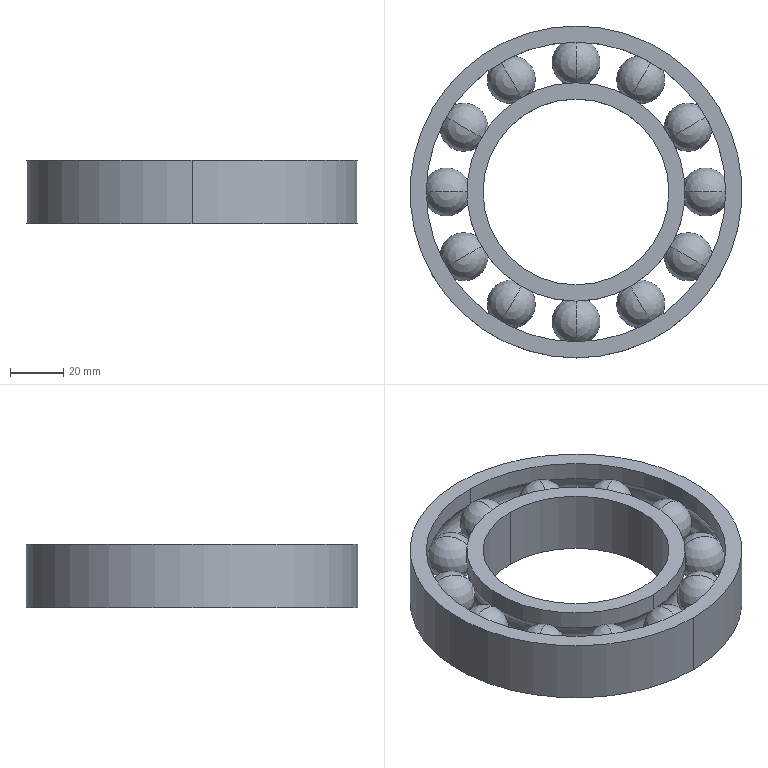Part | NX | features BREP 14 | 14 solids | 44 faces | box 125 x 125 x 24 mm | volume 122130 mm3 | sphere 24 | cylinder 12 | plane 4 | torus 4 | commonest cylinder face diameters 82.222 x4 112.778 x4 70 x2 125 x2
STEP:
#1=CARTESIAN_POINT('',(0.,62.5,-12.));
#2=VERTEX_POINT('',#1);
#3=CARTESIAN_POINT('',(0.,-62.5,-12.));
#4=VERTEX_POINT('',#3);
#5=CARTESIAN_POINT('',(0.,0.,-12.));
#6=DIRECTION('',(0.,0.,1.));
#7=DIRECTION('',(0.,1.,0.));
#8=AXIS2_PLACEMENT_3D('',#5,#6,#7);
#9=CIRCLE('',#8,62.5);
#10=EDGE_CURVE('',#2,#4,#9,.T.);
#11=ORIENTED_EDGE('',*,*,#10,.T.);
#12=CARTESIAN_POINT('',(0.,-62.5,12.));
#13=VERTEX_POINT('',#12);
#14=CARTESIAN_POINT('',(0.,-62.5,-12.));
#15=DIRECTION('',(0.,0.,1.));
#16=VECTOR('',#15,1000.);
#17=LINE('',#14,#16);
#18=EDGE_CURVE('',#4,#13,#17,.T.);
#19=ORIENTED_EDGE('',*,*,#18,.T.);
#20=CARTESIAN_POINT('',(0.,62.5,12.));
#21=VERTEX_POINT('',#20);
#22=CARTESIAN_POINT('',(0.,0.,12.));
#23=DIRECTION('',(0.,0.,1.));
#24=DIRECTION('',(0.,1.,0.));
#25=AXIS2_PLACEMENT_3D('',#22,#23,#24);
#26=CIRCLE('',#25,62.5);
#27=EDGE_CURVE('',#21,#13,#26,.T.);
#28=ORIENTED_EDGE('',*,*,#27,.F.);
#29=CARTESIAN_POINT('',(0.,62.5,-12.));
#30=DIRECTION('',(0.,0.,1.));
#31=VECTOR('',#30,1000.);
#32=LINE('',#29,#31);
#33=EDGE_CURVE('',#2,#21,#32,.T.);
#34=ORIENTED_EDGE('',*,*,#33,.F.);
#35=EDGE_LOOP('',(#11,#19,#28,#34));
#36=FACE_BOUND('',#35,.T.);
#37=CARTESIAN_POINT('',(0.,0.,13.2));
#38=DIRECTION('',(0.,0.,-1.));
#39=DIRECTION('',(0.,1.,0.));
#40=AXIS2_PLACEMENT_3D('',#37,#38,#39);
#41=CYLINDRICAL_SURFACE('',#40,62.5);
#42=ADVANCED_FACE('',(#36),#41,.T.);
#43=CARTESIAN_POINT('',(0.,0.,12.));
#44=DIRECTION('',(0.,0.,-1.));
#45=DIRECTION('',(0.,1.,0.));
#46=AXIS2_PLACEMENT_3D('',#43,#44,#45);
#47=CIRCLE('',#46,62.5);
#48=EDGE_CURVE('',#21,#13,#47,.T.);
#49=ORIENTED_EDGE('',*,*,#48,.T.);
#50=ORIENTED_EDGE('',*,*,#18,.F.);
#51=CARTESIAN_POINT('',(0.,0.,-12.));
#52=DIRECTION('',(0.,0.,-1.));
#53=DIRECTION('',(0.,1.,0.));
#54=AXIS2_PLACEMENT_3D('',#51,#52,#53);
#55=CIRCLE('',#54,62.5);
#56=EDGE_CURVE('',#2,#4,#55,.T.);
#57=ORIENTED_EDGE('',*,*,#56,.F.);
#58=ORIENTED_EDGE('',*,*,#33,.T.);
#59=EDGE_LOOP('',(#49,#50,#57,#58));
#60=FACE_BOUND('',#59,.T.);
#61=CARTESIAN_POINT('',(0.,0.,13.2));
#62=DIRECTION('',(0.,0.,-1.));
#63=DIRECTION('',(0.,1.,0.));
#64=AXIS2_PLACEMENT_3D('',#61,#62,#63);
#65=CYLINDRICAL_SURFACE('',#64,62.5);
#66=ADVANCED_FACE('',(#60),#65,.T.);
#67=ORIENTED_EDGE('',*,*,#10,.F.);
#68=ORIENTED_EDGE('',*,*,#56,.T.);
#69=EDGE_LOOP('',(#67,#68));
#70=FACE_BOUND('',#69,.T.);
#71=CARTESIAN_POINT('',(0.,56.389,-12.));
#72=VERTEX_POINT('',#71);
#73=CARTESIAN_POINT('',(0.,-56.389,-12.));
#74=VERTEX_POINT('',#73);
#75=CARTESIAN_POINT('',(0.,0.,-12.));
#76=DIRECTION('',(0.,0.,-1.));
#77=DIRECTION('',(0.,1.,0.));
#78=AXIS2_PLACEMENT_3D('',#75,#76,#77);
#79=CIRCLE('',#78,56.389);
#80=EDGE_CURVE('',#72,#74,#79,.T.);
#81=ORIENTED_EDGE('',*,*,#80,.F.);
#82=CARTESIAN_POINT('',(0.,0.,-12.));
#83=DIRECTION('',(0.,0.,1.));
#84=DIRECTION('',(0.,1.,0.));
#85=AXIS2_PLACEMENT_3D('',#82,#83,#84);
#86=CIRCLE('',#85,56.389);
#87=EDGE_CURVE('',#72,#74,#86,.T.);
#88=ORIENTED_EDGE('',*,*,#87,.T.);
#89=EDGE_LOOP('',(#81,#88));
#90=FACE_BOUND('',#89,.T.);
#91=CARTESIAN_POINT('',(0.,0.,-12.));
#92=DIRECTION('',(0.,0.,-1.));
#93=DIRECTION('',(0.,1.,0.));
#94=AXIS2_PLACEMENT_3D('',#91,#92,#93);
#95=PLANE('',#94);
#96=ADVANCED_FACE('',(#70,#90),#95,.T.);
#97=CARTESIAN_POINT('',(0.,56.389,-5.067));
#98=VERTEX_POINT('',#97);
#99=CARTESIAN_POINT('',(0.,-56.389,-5.067));
#100=VERTEX_POINT('',#99);
#101=CARTESIAN_POINT('',(0.,0.,-5.067));
#102=DIRECTION('',(0.,0.,1.));
#103=DIRECTION('',(0.,1.,0.));
#104=AXIS2_PLACEMENT_3D('',#101,#102,#103);
#105=CIRCLE('',#104,56.389);
#106=EDGE_CURVE('',#98,#100,#105,.T.);
#107=ORIENTED_EDGE('',*,*,#106,.T.);
#108=CARTESIAN_POINT('',(0.,-56.389,-5.067));
#109=DIRECTION('',(0.,0.,-1.));
#110=VECTOR('',#109,1000.);
#111=LINE('',#108,#110);
#112=EDGE_CURVE('',#100,#74,#111,.T.);
#113=ORIENTED_EDGE('',*,*,#112,.T.);
#114=ORIENTED_EDGE('',*,*,#87,.F.);
#115=CARTESIAN_POINT('',(0.,56.389,-5.067));
#116=DIRECTION('',(0.,0.,-1.));
#117=VECTOR('',#116,1000.);
#118=LINE('',#115,#117);
#119=EDGE_CURVE('',#98,#72,#118,.T.);
#120=ORIENTED_EDGE('',*,*,#119,.F.);
#121=EDGE_LOOP('',(#107,#113,#114,#120));
#122=FACE_BOUND('',#121,.T.);
#123=CARTESIAN_POINT('',(0.,0.,13.2));
#124=DIRECTION('',(0.,0.,-1.));
#125=DIRECTION('',(0.,1.,0.));
#126=AXIS2_PLACEMENT_3D('',#123,#124,#125);
#127=CYLINDRICAL_SURFACE('',#126,56.389);
#128=ADVANCED_FACE('',(#122),#127,.F.);
#129=ORIENTED_EDGE('',*,*,#80,.T.);
#130=ORIENTED_EDGE('',*,*,#112,.F.);
#131=CARTESIAN_POINT('',(0.,0.,-5.067));
#132=DIRECTION('',(0.,0.,-1.));
#133=DIRECTION('',(0.,1.,0.));
#134=AXIS2_PLACEMENT_3D('',#131,#132,#133);
#135=CIRCLE('',#134,56.389);
#136=EDGE_CURVE('',#98,#100,#135,.T.);
#137=ORIENTED_EDGE('',*,*,#136,.F.);
#138=ORIENTED_EDGE('',*,*,#119,.T.);
#139=EDGE_LOOP('',(#129,#130,#137,#138));
#140=FACE_BOUND('',#139,.T.);
#141=CARTESIAN_POINT('',(0.,0.,13.2));
#142=DIRECTION('',(0.,0.,-1.));
#143=DIRECTION('',(0.,1.,0.));
#144=AXIS2_PLACEMENT_3D('',#141,#142,#143);
#145=CYLINDRICAL_SURFACE('',#144,56.389);
#146=ADVANCED_FACE('',(#140),#145,.F.);
#147=ORIENTED_EDGE('',*,*,#136,.T.);
#148=CARTESIAN_POINT('',(0.,-56.389,5.067));
#149=VERTEX_POINT('',#148);
#150=CARTESIAN_POINT('',(0.,-48.75,0.));
#151=DIRECTION('',(1.,0.,0.));
#152=DIRECTION('',(0.,-0.8333,0.5528));
#153=AXIS2_PLACEMENT_3D('',#150,#151,#152);
#154=CIRCLE('',#153,9.167);
#155=EDGE_CURVE('',#100,#149,#154,.F.);
#156=ORIENTED_EDGE('',*,*,#155,.T.);
#157=CARTESIAN_POINT('',(0.,56.389,5.067));
#158=VERTEX_POINT('',#157);
#159=CARTESIAN_POINT('',(0.,0.,5.067));
#160=DIRECTION('',(0.,0.,-1.));
#161=DIRECTION('',(0.,1.,0.));
#162=AXIS2_PLACEMENT_3D('',#159,#160,#161);
#163=CIRCLE('',#162,56.389);
#164=EDGE_CURVE('',#158,#149,#163,.T.);
#165=ORIENTED_EDGE('',*,*,#164,.F.);
#166=CARTESIAN_POINT('',(0.,48.75,0.));
#167=DIRECTION('',(-1.,0.,0.));
#168=DIRECTION('',(0.,0.8333,0.5528));
#169=AXIS2_PLACEMENT_3D('',#166,#167,#168);
#170=CIRCLE('',#169,9.167);
#171=EDGE_CURVE('',#98,#158,#170,.F.);
#172=ORIENTED_EDGE('',*,*,#171,.F.);
#173=EDGE_LOOP('',(#147,#156,#165,#172));
#174=FACE_BOUND('',#173,.T.);
#175=CARTESIAN_POINT('',(0.,0.,0.));
#176=DIRECTION('',(0.,0.,-1.));
#177=DIRECTION('',(0.,1.,0.));
#178=AXIS2_PLACEMENT_3D('',#175,#176,#177);
#179=TOROIDAL_SURFACE('',#178,48.75,9.167);
#180=ADVANCED_FACE('',(#174),#179,.F.);
#181=CARTESIAN_POINT('',(0.,0.,5.067));
#182=DIRECTION('',(0.,0.,1.));
#183=DIRECTION('',(0.,1.,0.));
#184=AXIS2_PLACEMENT_3D('',#181,#182,#183);
#185=CIRCLE('',#184,56.389);
#186=EDGE_CURVE('',#158,#149,#185,.T.);
#187=ORIENTED_EDGE('',*,*,#186,.T.);
#188=ORIENTED_EDGE('',*,*,#155,.F.);
#189=ORIENTED_EDGE('',*,*,#106,.F.);
#190=ORIENTED_EDGE('',*,*,#171,.T.);
#191=EDGE_LOOP('',(#187,#188,#189,#190));
#192=FACE_BOUND('',#191,.T.);
#193=CARTESIAN_POINT('',(0.,0.,0.));
#194=DIRECTION('',(0.,0.,-1.));
#195=DIRECTION('',(0.,1.,0.));
#196=AXIS2_PLACEMENT_3D('',#193,#194,#195);
#197=TOROIDAL_SURFACE('',#196,48.75,9.167);
#198=ADVANCED_FACE('',(#192),#197,.F.);
#199=CARTESIAN_POINT('',(0.,56.389,12.));
#200=VERTEX_POINT('',#199);
#201=CARTESIAN_POINT('',(0.,-56.389,12.));
#202=VERTEX_POINT('',#201);
#203=CARTESIAN_POINT('',(0.,0.,12.));
#204=DIRECTION('',(0.,0.,1.));
#205=DIRECTION('',(0.,1.,0.));
#206=AXIS2_PLACEMENT_3D('',#203,#204,#205);
#207=CIRCLE('',#206,56.389);
#208=EDGE_CURVE('',#200,#202,#207,.T.);
#209=ORIENTED_EDGE('',*,*,#208,.T.);
#210=CARTESIAN_POINT('',(0.,-56.389,12.));
#211=DIRECTION('',(0.,0.,-1.));
#212=VECTOR('',#211,1000.);
#213=LINE('',#210,#212);
#214=EDGE_CURVE('',#202,#149,#213,.T.);
#215=ORIENTED_EDGE('',*,*,#214,.T.);
#216=ORIENTED_EDGE('',*,*,#186,.F.);
#217=CARTESIAN_POINT('',(0.,56.389,12.));
#218=DIRECTION('',(0.,0.,-1.));
#219=VECTOR('',#218,1000.);
#220=LINE('',#217,#219);
#221=EDGE_CURVE('',#200,#158,#220,.T.);
#222=ORIENTED_EDGE('',*,*,#221,.F.);
#223=EDGE_LOOP('',(#209,#215,#216,#222));
#224=FACE_BOUND('',#223,.T.);
#225=CARTESIAN_POINT('',(0.,0.,13.2));
#226=DIRECTION('',(0.,0.,-1.));
#227=DIRECTION('',(0.,1.,0.));
#228=AXIS2_PLACEMENT_3D('',#225,#226,#227);
#229=CYLINDRICAL_SURFACE('',#228,56.389);
#230=ADVANCED_FACE('',(#224),#229,.F.);
#231=ORIENTED_EDGE('',*,*,#164,.T.);
#232=ORIENTED_EDGE('',*,*,#214,.F.);
#233=CARTESIAN_POINT('',(0.,0.,12.));
#234=DIRECTION('',(0.,0.,-1.));
#235=DIRECTION('',(0.,1.,0.));
#236=AXIS2_PLACEMENT_3D('',#233,#234,#235);
#237=CIRCLE('',#236,56.389);
#238=EDGE_CURVE('',#200,#202,#237,.T.);
#239=ORIENTED_EDGE('',*,*,#238,.F.);
#240=ORIENTED_EDGE('',*,*,#221,.T.);
#241=EDGE_LOOP('',(#231,#232,#239,#240));
#242=FACE_BOUND('',#241,.T.);
#243=CARTESIAN_POINT('',(0.,0.,13.2));
#244=DIRECTION('',(0.,0.,-1.));
#245=DIRECTION('',(0.,1.,0.));
#246=AXIS2_PLACEMENT_3D('',#243,#244,#245);
#247=CYLINDRICAL_SURFACE('',#246,56.389);
#248=ADVANCED_FACE('',(#242),#247,.F.);
#249=ORIENTED_EDGE('',*,*,#48,.F.);
#250=ORIENTED_EDGE('',*,*,#27,.T.);
#251=EDGE_LOOP('',(#249,#250));
#252=FACE_BOUND('',#251,.T.);
#253=ORIENTED_EDGE('',*,*,#208,.F.);
#254=ORIENTED_EDGE('',*,*,#238,.T.);
#255=EDGE_LOOP('',(#253,#254));
#256=FACE_BOUND('',#255,.T.);
#257=CARTESIAN_POINT('',(0.,0.,12.));
#258=DIRECTION('',(0.,0.,-1.));
#259=DIRECTION('',(0.,1.,0.));
#260=AXIS2_PLACEMENT_3D('',#257,#258,#259);
#261=PLANE('',#260);
#262=ADVANCED_FACE('',(#252,#256),#261,.F.);
#263=CLOSED_SHELL('',(#42,#66,#96,#128,#146,#180,#198,#230,#248,#262));
#264=MANIFOLD_SOLID_BREP('',#263);
#265=CARTESIAN_POINT('',(48.75,0.,9.167));
#266=VERTEX_POINT('',#265);
#267=CARTESIAN_POINT('',(48.75,0.,-9.167));
#268=VERTEX_POINT('',#267);
#269=CARTESIAN_POINT('',(48.75,0.,0.));
#270=DIRECTION('',(0.,1.,0.));
#271=DIRECTION('',(0.,0.,-1.));
#272=AXIS2_PLACEMENT_3D('',#269,#270,#271);
#273=CIRCLE('',#272,9.167);
#274=EDGE_CURVE('',#266,#268,#273,.F.);
#275=ORIENTED_EDGE('',*,*,#274,.T.);
#276=CARTESIAN_POINT('',(48.75,0.,0.));
#277=DIRECTION('',(0.,-1.,0.));
#278=DIRECTION('',(0.,0.,-1.));
#279=AXIS2_PLACEMENT_3D('',#276,#277,#278);
#280=CIRCLE('',#279,9.167);
#281=EDGE_CURVE('',#266,#268,#280,.F.);
#282=ORIENTED_EDGE('',*,*,#281,.F.);
#283=EDGE_LOOP('',(#275,#282));
#284=FACE_BOUND('',#283,.T.);
#285=CARTESIAN_POINT('',(48.75,0.,0.));
#286=DIRECTION('',(0.,0.,-1.));
#287=DIRECTION('',(1.,0.,0.));
#288=AXIS2_PLACEMENT_3D('',#285,#286,#287);
#289=SPHERICAL_SURFACE('',#288,9.167);
#290=ADVANCED_FACE('',(#284),#289,.T.);
#291=ORIENTED_EDGE('',*,*,#274,.F.);
#292=ORIENTED_EDGE('',*,*,#281,.T.);
#293=EDGE_LOOP('',(#291,#292));
#294=FACE_BOUND('',#293,.T.);
#295=CARTESIAN_POINT('',(48.75,0.,0.));
#296=DIRECTION('',(0.,0.,-1.));
#297=DIRECTION('',(1.,0.,0.));
#298=AXIS2_PLACEMENT_3D('',#295,#296,#297);
#299=SPHERICAL_SURFACE('',#298,9.167);
#300=ADVANCED_FACE('',(#294),#299,.T.);
#301=CLOSED_SHELL('',(#290,#300));
#302=MANIFOLD_SOLID_BREP('',#301);
#303=CARTESIAN_POINT('',(-42.219,-24.375,-9.167));
#304=VERTEX_POINT('',#303);
#305=CARTESIAN_POINT('',(-42.219,-24.375,9.167));
#306=VERTEX_POINT('',#305);
#307=CARTESIAN_POINT('',(-42.219,-24.375,0.));
#308=DIRECTION('',(0.5,-0.866,0.));
#309=DIRECTION('',(0.,0.,-1.));
#310=AXIS2_PLACEMENT_3D('',#307,#308,#309);
#311=CIRCLE('',#310,9.167);
#312=EDGE_CURVE('',#304,#306,#311,.T.);
#313=ORIENTED_EDGE('',*,*,#312,.F.);
#314=CARTESIAN_POINT('',(-42.219,-24.375,0.));
#315=DIRECTION('',(-0.5,0.866,0.));
#316=DIRECTION('',(0.,0.,-1.));
#317=AXIS2_PLACEMENT_3D('',#314,#315,#316);
#318=CIRCLE('',#317,9.167);
#319=EDGE_CURVE('',#304,#306,#318,.T.);
#320=ORIENTED_EDGE('',*,*,#319,.T.);
#321=EDGE_LOOP('',(#313,#320));
#322=FACE_BOUND('',#321,.T.);
#323=CARTESIAN_POINT('',(-42.219,-24.375,0.));
#324=DIRECTION('',(0.,0.,-1.));
#325=DIRECTION('',(-0.866,-0.5,0.));
#326=AXIS2_PLACEMENT_3D('',#323,#324,#325);
#327=SPHERICAL_SURFACE('',#326,9.167);
#328=ADVANCED_FACE('',(#322),#327,.T.);
#329=ORIENTED_EDGE('',*,*,#312,.T.);
#330=ORIENTED_EDGE('',*,*,#319,.F.);
#331=EDGE_LOOP('',(#329,#330));
#332=FACE_BOUND('',#331,.T.);
#333=CARTESIAN_POINT('',(-42.219,-24.375,0.));
#334=DIRECTION('',(0.,0.,-1.));
#335=DIRECTION('',(-0.866,-0.5,0.));
#336=AXIS2_PLACEMENT_3D('',#333,#334,#335);
#337=SPHERICAL_SURFACE('',#336,9.167);
#338=ADVANCED_FACE('',(#332),#337,.T.);
#339=CLOSED_SHELL('',(#328,#338));
#340=MANIFOLD_SOLID_BREP('',#339);
#341=CARTESIAN_POINT('',(0.,41.111,5.067));
#342=VERTEX_POINT('',#341);
#343=CARTESIAN_POINT('',(0.,-41.111,5.067));
#344=VERTEX_POINT('',#343);
#345=CARTESIAN_POINT('',(0.,0.,5.067));
#346=DIRECTION('',(0.,0.,1.));
#347=DIRECTION('',(0.,1.,0.));
#348=AXIS2_PLACEMENT_3D('',#345,#346,#347);
#349=CIRCLE('',#348,41.111);
#350=EDGE_CURVE('',#342,#344,#349,.T.);
#351=ORIENTED_EDGE('',*,*,#350,.T.);
#352=CARTESIAN_POINT('',(0.,-41.111,12.));
#353=VERTEX_POINT('',#352);
#354=CARTESIAN_POINT('',(0.,-41.111,5.067));
#355=DIRECTION('',(0.,0.,1.));
#356=VECTOR('',#355,1000.);
#357=LINE('',#354,#356);
#358=EDGE_CURVE('',#344,#353,#357,.T.);
#359=ORIENTED_EDGE('',*,*,#358,.T.);
#360=CARTESIAN_POINT('',(0.,41.111,12.));
#361=VERTEX_POINT('',#360);
#362=CARTESIAN_POINT('',(0.,0.,12.));
#363=DIRECTION('',(0.,0.,1.));
#364=DIRECTION('',(0.,1.,0.));
#365=AXIS2_PLACEMENT_3D('',#362,#363,#364);
#366=CIRCLE('',#365,41.111);
#367=EDGE_CURVE('',#361,#353,#366,.T.);
#368=ORIENTED_EDGE('',*,*,#367,.F.);
#369=CARTESIAN_POINT('',(0.,41.111,5.067));
#370=DIRECTION('',(0.,0.,1.));
#371=VECTOR('',#370,1000.);
#372=LINE('',#369,#371);
#373=EDGE_CURVE('',#342,#361,#372,.T.);
#374=ORIENTED_EDGE('',*,*,#373,.F.);
#375=EDGE_LOOP('',(#351,#359,#368,#374));
#376=FACE_BOUND('',#375,.T.);
#377=CARTESIAN_POINT('',(0.,0.,13.2));
#378=DIRECTION('',(0.,0.,-1.));
#379=DIRECTION('',(0.,1.,0.));
#380=AXIS2_PLACEMENT_3D('',#377,#378,#379);
#381=CYLINDRICAL_SURFACE('',#380,41.111);
#382=ADVANCED_FACE('',(#376),#381,.T.);
#383=CARTESIAN_POINT('',(0.,0.,12.));
#384=DIRECTION('',(0.,0.,-1.));
#385=DIRECTION('',(0.,1.,0.));
#386=AXIS2_PLACEMENT_3D('',#383,#384,#385);
#387=CIRCLE('',#386,41.111);
#388=EDGE_CURVE('',#361,#353,#387,.T.);
#389=ORIENTED_EDGE('',*,*,#388,.T.);
#390=ORIENTED_EDGE('',*,*,#358,.F.);
#391=CARTESIAN_POINT('',(0.,0.,5.067));
#392=DIRECTION('',(0.,0.,-1.));
#393=DIRECTION('',(0.,1.,0.));
#394=AXIS2_PLACEMENT_3D('',#391,#392,#393);
#395=CIRCLE('',#394,41.111);
#396=EDGE_CURVE('',#342,#344,#395,.T.);
#397=ORIENTED_EDGE('',*,*,#396,.F.);
#398=ORIENTED_EDGE('',*,*,#373,.T.);
#399=EDGE_LOOP('',(#389,#390,#397,#398));
#400=FACE_BOUND('',#399,.T.);
#401=CARTESIAN_POINT('',(0.,0.,13.2));
#402=DIRECTION('',(0.,0.,-1.));
#403=DIRECTION('',(0.,1.,0.));
#404=AXIS2_PLACEMENT_3D('',#401,#402,#403);
#405=CYLINDRICAL_SURFACE('',#404,41.111);
#406=ADVANCED_FACE('',(#400),#405,.T.);
#407=ORIENTED_EDGE('',*,*,#396,.T.);
#408=CARTESIAN_POINT('',(0.,-41.111,-5.067));
#409=VERTEX_POINT('',#408);
#410=CARTESIAN_POINT('',(0.,-48.75,0.));
#411=DIRECTION('',(1.,0.,0.));
#412=DIRECTION('',(0.,0.8333,-0.5528));
#413=AXIS2_PLACEMENT_3D('',#410,#411,#412);
#414=CIRCLE('',#413,9.167);
#415=EDGE_CURVE('',#344,#409,#414,.F.);
#416=ORIENTED_EDGE('',*,*,#415,.T.);
#417=CARTESIAN_POINT('',(0.,41.111,-5.067));
#418=VERTEX_POINT('',#417);
#419=CARTESIAN_POINT('',(0.,0.,-5.067));
#420=DIRECTION('',(0.,0.,-1.));
#421=DIRECTION('',(0.,1.,0.));
#422=AXIS2_PLACEMENT_3D('',#419,#420,#421);
#423=CIRCLE('',#422,41.111);
#424=EDGE_CURVE('',#418,#409,#423,.T.);
#425=ORIENTED_EDGE('',*,*,#424,.F.);
#426=CARTESIAN_POINT('',(0.,48.75,0.));
#427=DIRECTION('',(-1.,0.,0.));
#428=DIRECTION('',(0.,-0.8333,-0.5528));
#429=AXIS2_PLACEMENT_3D('',#426,#427,#428);
#430=CIRCLE('',#429,9.167);
#431=EDGE_CURVE('',#342,#418,#430,.F.);
#432=ORIENTED_EDGE('',*,*,#431,.F.);
#433=EDGE_LOOP('',(#407,#416,#425,#432));
#434=FACE_BOUND('',#433,.T.);
#435=CARTESIAN_POINT('',(0.,0.,0.));
#436=DIRECTION('',(0.,0.,-1.));
#437=DIRECTION('',(0.,1.,0.));
#438=AXIS2_PLACEMENT_3D('',#435,#436,#437);
#439=TOROIDAL_SURFACE('',#438,48.75,9.167);
#440=ADVANCED_FACE('',(#434),#439,.F.);
#441=CARTESIAN_POINT('',(0.,0.,-5.067));
#442=DIRECTION('',(0.,0.,1.));
#443=DIRECTION('',(0.,1.,0.));
#444=AXIS2_PLACEMENT_3D('',#441,#442,#443);
#445=CIRCLE('',#444,41.111);
#446=EDGE_CURVE('',#418,#409,#445,.T.);
#447=ORIENTED_EDGE('',*,*,#446,.T.);
#448=ORIENTED_EDGE('',*,*,#415,.F.);
#449=ORIENTED_EDGE('',*,*,#350,.F.);
#450=ORIENTED_EDGE('',*,*,#431,.T.);
#451=EDGE_LOOP('',(#447,#448,#449,#450));
#452=FACE_BOUND('',#451,.T.);
#453=CARTESIAN_POINT('',(0.,0.,0.));
#454=DIRECTION('',(0.,0.,-1.));
#455=DIRECTION('',(0.,1.,0.));
#456=AXIS2_PLACEMENT_3D('',#453,#454,#455);
#457=TOROIDAL_SURFACE('',#456,48.75,9.167);
#458=ADVANCED_FACE('',(#452),#457,.F.);
#459=CARTESIAN_POINT('',(0.,41.111,-12.));
#460=VERTEX_POINT('',#459);
#461=CARTESIAN_POINT('',(0.,-41.111,-12.));
#462=VERTEX_POINT('',#461);
#463=CARTESIAN_POINT('',(0.,0.,-12.));
#464=DIRECTION('',(0.,0.,1.));
#465=DIRECTION('',(0.,1.,0.));
#466=AXIS2_PLACEMENT_3D('',#463,#464,#465);
#467=CIRCLE('',#466,41.111);
#468=EDGE_CURVE('',#460,#462,#467,.T.);
#469=ORIENTED_EDGE('',*,*,#468,.T.);
#470=CARTESIAN_POINT('',(0.,-41.111,-12.));
#471=DIRECTION('',(0.,0.,1.));
#472=VECTOR('',#471,1000.);
#473=LINE('',#470,#472);
#474=EDGE_CURVE('',#462,#409,#473,.T.);
#475=ORIENTED_EDGE('',*,*,#474,.T.);
#476=ORIENTED_EDGE('',*,*,#446,.F.);
#477=CARTESIAN_POINT('',(0.,41.111,-12.));
#478=DIRECTION('',(0.,0.,1.));
#479=VECTOR('',#478,1000.);
#480=LINE('',#477,#479);
#481=EDGE_CURVE('',#460,#418,#480,.T.);
#482=ORIENTED_EDGE('',*,*,#481,.F.);
#483=EDGE_LOOP('',(#469,#475,#476,#482));
#484=FACE_BOUND('',#483,.T.);
#485=CARTESIAN_POINT('',(0.,0.,13.2));
#486=DIRECTION('',(0.,0.,-1.));
#487=DIRECTION('',(0.,1.,0.));
#488=AXIS2_PLACEMENT_3D('',#485,#486,#487);
#489=CYLINDRICAL_SURFACE('',#488,41.111);
#490=ADVANCED_FACE('',(#484),#489,.T.);
#491=ORIENTED_EDGE('',*,*,#424,.T.);
#492=ORIENTED_EDGE('',*,*,#474,.F.);
#493=CARTESIAN_POINT('',(0.,0.,-12.));
#494=DIRECTION('',(0.,0.,-1.));
#495=DIRECTION('',(0.,1.,0.));
#496=AXIS2_PLACEMENT_3D('',#493,#494,#495);
#497=CIRCLE('',#496,41.111);
#498=EDGE_CURVE('',#460,#462,#497,.T.);
#499=ORIENTED_EDGE('',*,*,#498,.F.);
#500=ORIENTED_EDGE('',*,*,#481,.T.);
#501=EDGE_LOOP('',(#491,#492,#499,#500));
#502=FACE_BOUND('',#501,.T.);
#503=CARTESIAN_POINT('',(0.,0.,13.2));
#504=DIRECTION('',(0.,0.,-1.));
#505=DIRECTION('',(0.,1.,0.));
#506=AXIS2_PLACEMENT_3D('',#503,#504,#505);
#507=CYLINDRICAL_SURFACE('',#506,41.111);
#508=ADVANCED_FACE('',(#502),#507,.T.);
#509=ORIENTED_EDGE('',*,*,#468,.F.);
#510=ORIENTED_EDGE('',*,*,#498,.T.);
#511=EDGE_LOOP('',(#509,#510));
#512=FACE_BOUND('',#511,.T.);
#513=CARTESIAN_POINT('',(0.,35.,-12.));
#514=VERTEX_POINT('',#513);
#515=CARTESIAN_POINT('',(0.,-35.,-12.));
#516=VERTEX_POINT('',#515);
#517=CARTESIAN_POINT('',(0.,0.,-12.));
#518=DIRECTION('',(0.,0.,-1.));
#519=DIRECTION('',(0.,1.,0.));
#520=AXIS2_PLACEMENT_3D('',#517,#518,#519);
#521=CIRCLE('',#520,35.);
#522=EDGE_CURVE('',#514,#516,#521,.T.);
#523=ORIENTED_EDGE('',*,*,#522,.F.);
#524=CARTESIAN_POINT('',(0.,0.,-12.));
#525=DIRECTION('',(0.,0.,1.));
#526=DIRECTION('',(0.,1.,0.));
#527=AXIS2_PLACEMENT_3D('',#524,#525,#526);
#528=CIRCLE('',#527,35.);
#529=EDGE_CURVE('',#514,#516,#528,.T.);
#530=ORIENTED_EDGE('',*,*,#529,.T.);
#531=EDGE_LOOP('',(#523,#530));
#532=FACE_BOUND('',#531,.T.);
#533=CARTESIAN_POINT('',(0.,0.,-12.));
#534=DIRECTION('',(0.,0.,-1.));
#535=DIRECTION('',(0.,1.,0.));
#536=AXIS2_PLACEMENT_3D('',#533,#534,#535);
#537=PLANE('',#536);
#538=ADVANCED_FACE('',(#512,#532),#537,.T.);
#539=CARTESIAN_POINT('',(0.,35.,12.));
#540=VERTEX_POINT('',#539);
#541=CARTESIAN_POINT('',(0.,-35.,12.));
#542=VERTEX_POINT('',#541);
#543=CARTESIAN_POINT('',(0.,0.,12.));
#544=DIRECTION('',(0.,0.,1.));
#545=DIRECTION('',(0.,1.,0.));
#546=AXIS2_PLACEMENT_3D('',#543,#544,#545);
#547=CIRCLE('',#546,35.);
#548=EDGE_CURVE('',#540,#542,#547,.T.);
#549=ORIENTED_EDGE('',*,*,#548,.T.);
#550=CARTESIAN_POINT('',(0.,-35.,12.));
#551=DIRECTION('',(0.,0.,-1.));
#552=VECTOR('',#551,1000.);
#553=LINE('',#550,#552);
#554=EDGE_CURVE('',#542,#516,#553,.T.);
#555=ORIENTED_EDGE('',*,*,#554,.T.);
#556=ORIENTED_EDGE('',*,*,#529,.F.);
#557=CARTESIAN_POINT('',(0.,35.,12.));
#558=DIRECTION('',(0.,0.,-1.));
#559=VECTOR('',#558,1000.);
#560=LINE('',#557,#559);
#561=EDGE_CURVE('',#540,#514,#560,.T.);
#562=ORIENTED_EDGE('',*,*,#561,.F.);
#563=EDGE_LOOP('',(#549,#555,#556,#562));
#564=FACE_BOUND('',#563,.T.);
#565=CARTESIAN_POINT('',(0.,0.,13.2));
#566=DIRECTION('',(0.,0.,-1.));
#567=DIRECTION('',(0.,1.,0.));
#568=AXIS2_PLACEMENT_3D('',#565,#566,#567);
#569=CYLINDRICAL_SURFACE('',#568,35.);
#570=ADVANCED_FACE('',(#564),#569,.F.);
#571=ORIENTED_EDGE('',*,*,#522,.T.);
#572=ORIENTED_EDGE('',*,*,#554,.F.);
#573=CARTESIAN_POINT('',(0.,0.,12.));
#574=DIRECTION('',(0.,0.,-1.));
#575=DIRECTION('',(0.,1.,0.));
#576=AXIS2_PLACEMENT_3D('',#573,#574,#575);
#577=CIRCLE('',#576,35.);
#578=EDGE_CURVE('',#540,#542,#577,.T.);
#579=ORIENTED_EDGE('',*,*,#578,.F.);
#580=ORIENTED_EDGE('',*,*,#561,.T.);
#581=EDGE_LOOP('',(#571,#572,#579,#580));
#582=FACE_BOUND('',#581,.T.);
#583=CARTESIAN_POINT('',(0.,0.,13.2));
#584=DIRECTION('',(0.,0.,-1.));
#585=DIRECTION('',(0.,1.,0.));
#586=AXIS2_PLACEMENT_3D('',#583,#584,#585);
#587=CYLINDRICAL_SURFACE('',#586,35.);
#588=ADVANCED_FACE('',(#582),#587,.F.);
#589=ORIENTED_EDGE('',*,*,#388,.F.);
#590=ORIENTED_EDGE('',*,*,#367,.T.);
#591=EDGE_LOOP('',(#589,#590));
#592=FACE_BOUND('',#591,.T.);
#593=ORIENTED_EDGE('',*,*,#548,.F.);
#594=ORIENTED_EDGE('',*,*,#578,.T.);
#595=EDGE_LOOP('',(#593,#594));
#596=FACE_BOUND('',#595,.T.);
#597=CARTESIAN_POINT('',(0.,0.,12.));
#598=DIRECTION('',(0.,0.,-1.));
#599=DIRECTION('',(0.,1.,0.));
#600=AXIS2_PLACEMENT_3D('',#597,#598,#599);
#601=PLANE('',#600);
#602=ADVANCED_FACE('',(#592,#596),#601,.F.);
#603=CLOSED_SHELL('',(#382,#406,#440,#458,#490,#508,#538,#570,#588,#602));
#604=MANIFOLD_SOLID_BREP('',#603);
#605=CARTESIAN_POINT('',(-48.75,0.,-9.167));
#606=VERTEX_POINT('',#605);
#607=CARTESIAN_POINT('',(-48.75,0.,9.167));
#608=VERTEX_POINT('',#607);
#609=CARTESIAN_POINT('',(-48.75,0.,0.));
#610=DIRECTION('',(0.,-1.,0.));
#611=DIRECTION('',(0.,0.,-1.));
#612=AXIS2_PLACEMENT_3D('',#609,#610,#611);
#613=CIRCLE('',#612,9.167);
#614=EDGE_CURVE('',#606,#608,#613,.T.);
#615=ORIENTED_EDGE('',*,*,#614,.F.);
#616=CARTESIAN_POINT('',(-48.75,0.,0.));
#617=DIRECTION('',(0.,1.,0.));
#618=DIRECTION('',(0.,0.,-1.));
#619=AXIS2_PLACEMENT_3D('',#616,#617,#618);
#620=CIRCLE('',#619,9.167);
#621=EDGE_CURVE('',#606,#608,#620,.T.);
#622=ORIENTED_EDGE('',*,*,#621,.T.);
#623=EDGE_LOOP('',(#615,#622));
#624=FACE_BOUND('',#623,.T.);
#625=CARTESIAN_POINT('',(-48.75,0.,0.));
#626=DIRECTION('',(0.,0.,-1.));
#627=DIRECTION('',(-1.,0.,0.));
#628=AXIS2_PLACEMENT_3D('',#625,#626,#627);
#629=SPHERICAL_SURFACE('',#628,9.167);
#630=ADVANCED_FACE('',(#624),#629,.T.);
#631=ORIENTED_EDGE('',*,*,#614,.T.);
#632=ORIENTED_EDGE('',*,*,#621,.F.);
#633=EDGE_LOOP('',(#631,#632));
#634=FACE_BOUND('',#633,.T.);
#635=CARTESIAN_POINT('',(-48.75,0.,0.));
#636=DIRECTION('',(0.,0.,-1.));
#637=DIRECTION('',(-1.,0.,0.));
#638=AXIS2_PLACEMENT_3D('',#635,#636,#637);
#639=SPHERICAL_SURFACE('',#638,9.167);
#640=ADVANCED_FACE('',(#634),#639,.T.);
#641=CLOSED_SHELL('',(#630,#640));
#642=MANIFOLD_SOLID_BREP('',#641);
#643=CARTESIAN_POINT('',(-24.375,42.219,-9.167));
#644=VERTEX_POINT('',#643);
#645=CARTESIAN_POINT('',(-24.375,42.219,9.167));
#646=VERTEX_POINT('',#645);
#647=CARTESIAN_POINT('',(-24.375,42.219,0.));
#648=DIRECTION('',(-0.866,-0.5,0.));
#649=DIRECTION('',(0.,0.,-1.));
#650=AXIS2_PLACEMENT_3D('',#647,#648,#649);
#651=CIRCLE('',#650,9.167);
#652=EDGE_CURVE('',#644,#646,#651,.T.);
#653=ORIENTED_EDGE('',*,*,#652,.F.);
#654=CARTESIAN_POINT('',(-24.375,42.219,0.));
#655=DIRECTION('',(0.866,0.5,0.));
#656=DIRECTION('',(0.,0.,-1.));
#657=AXIS2_PLACEMENT_3D('',#654,#655,#656);
#658=CIRCLE('',#657,9.167);
#659=EDGE_CURVE('',#644,#646,#658,.T.);
#660=ORIENTED_EDGE('',*,*,#659,.T.);
#661=EDGE_LOOP('',(#653,#660));
#662=FACE_BOUND('',#661,.T.);
#663=CARTESIAN_POINT('',(-24.375,42.219,0.));
#664=DIRECTION('',(0.,0.,-1.));
#665=DIRECTION('',(-0.5,0.866,0.));
#666=AXIS2_PLACEMENT_3D('',#663,#664,#665);
#667=SPHERICAL_SURFACE('',#666,9.167);
#668=ADVANCED_FACE('',(#662),#667,.T.);
#669=ORIENTED_EDGE('',*,*,#652,.T.);
#670=ORIENTED_EDGE('',*,*,#659,.F.);
#671=EDGE_LOOP('',(#669,#670));
#672=FACE_BOUND('',#671,.T.);
#673=CARTESIAN_POINT('',(-24.375,42.219,0.));
#674=DIRECTION('',(0.,0.,-1.));
#675=DIRECTION('',(-0.5,0.866,0.));
#676=AXIS2_PLACEMENT_3D('',#673,#674,#675);
#677=SPHERICAL_SURFACE('',#676,9.167);
#678=ADVANCED_FACE('',(#672),#677,.T.);
#679=CLOSED_SHELL('',(#668,#678));
#680=MANIFOLD_SOLID_BREP('',#679);
#681=CARTESIAN_POINT('',(-24.375,-42.219,-9.167));
#682=VERTEX_POINT('',#681);
#683=CARTESIAN_POINT('',(-24.375,-42.219,9.167));
#684=VERTEX_POINT('',#683);
#685=CARTESIAN_POINT('',(-24.375,-42.219,0.));
#686=DIRECTION('',(0.866,-0.5,0.));
#687=DIRECTION('',(0.,0.,-1.));
#688=AXIS2_PLACEMENT_3D('',#685,#686,#687);
#689=CIRCLE('',#688,9.167);
#690=EDGE_CURVE('',#682,#684,#689,.T.);
#691=ORIENTED_EDGE('',*,*,#690,.F.);
#692=CARTESIAN_POINT('',(-24.375,-42.219,0.));
#693=DIRECTION('',(-0.866,0.5,0.));
#694=DIRECTION('',(0.,0.,-1.));
#695=AXIS2_PLACEMENT_3D('',#692,#693,#694);
#696=CIRCLE('',#695,9.167);
#697=EDGE_CURVE('',#682,#684,#696,.T.);
#698=ORIENTED_EDGE('',*,*,#697,.T.);
#699=EDGE_LOOP('',(#691,#698));
#700=FACE_BOUND('',#699,.T.);
#701=CARTESIAN_POINT('',(-24.375,-42.219,0.));
#702=DIRECTION('',(0.,0.,-1.));
#703=DIRECTION('',(-0.5,-0.866,0.));
#704=AXIS2_PLACEMENT_3D('',#701,#702,#703);
#705=SPHERICAL_SURFACE('',#704,9.167);
#706=ADVANCED_FACE('',(#700),#705,.T.);
#707=ORIENTED_EDGE('',*,*,#690,.T.);
#708=ORIENTED_EDGE('',*,*,#697,.F.);
#709=EDGE_LOOP('',(#707,#708));
#710=FACE_BOUND('',#709,.T.);
#711=CARTESIAN_POINT('',(-24.375,-42.219,0.));
#712=DIRECTION('',(0.,0.,-1.));
#713=DIRECTION('',(-0.5,-0.866,0.));
#714=AXIS2_PLACEMENT_3D('',#711,#712,#713);
#715=SPHERICAL_SURFACE('',#714,9.167);
#716=ADVANCED_FACE('',(#710),#715,.T.);
#717=CLOSED_SHELL('',(#706,#716));
#718=MANIFOLD_SOLID_BREP('',#717);
#719=CARTESIAN_POINT('',(-42.219,24.375,-9.167));
#720=VERTEX_POINT('',#719);
#721=CARTESIAN_POINT('',(-42.219,24.375,9.167));
#722=VERTEX_POINT('',#721);
#723=CARTESIAN_POINT('',(-42.219,24.375,0.));
#724=DIRECTION('',(-0.5,-0.866,0.));
#725=DIRECTION('',(0.,0.,-1.));
#726=AXIS2_PLACEMENT_3D('',#723,#724,#725);
#727=CIRCLE('',#726,9.167);
#728=EDGE_CURVE('',#720,#722,#727,.T.);
#729=ORIENTED_EDGE('',*,*,#728,.F.);
#730=CARTESIAN_POINT('',(-42.219,24.375,0.));
#731=DIRECTION('',(0.5,0.866,0.));
#732=DIRECTION('',(0.,0.,-1.));
#733=AXIS2_PLACEMENT_3D('',#730,#731,#732);
#734=CIRCLE('',#733,9.167);
#735=EDGE_CURVE('',#720,#722,#734,.T.);
#736=ORIENTED_EDGE('',*,*,#735,.T.);
#737=EDGE_LOOP('',(#729,#736));
#738=FACE_BOUND('',#737,.T.);
#739=CARTESIAN_POINT('',(-42.219,24.375,0.));
#740=DIRECTION('',(0.,0.,-1.));
#741=DIRECTION('',(-0.866,0.5,0.));
#742=AXIS2_PLACEMENT_3D('',#739,#740,#741);
#743=SPHERICAL_SURFACE('',#742,9.167);
#744=ADVANCED_FACE('',(#738),#743,.T.);
#745=ORIENTED_EDGE('',*,*,#728,.T.);
#746=ORIENTED_EDGE('',*,*,#735,.F.);
#747=EDGE_LOOP('',(#745,#746));
#748=FACE_BOUND('',#747,.T.);
#749=CARTESIAN_POINT('',(-42.219,24.375,0.));
#750=DIRECTION('',(0.,0.,-1.));
#751=DIRECTION('',(-0.866,0.5,0.));
#752=AXIS2_PLACEMENT_3D('',#749,#750,#751);
#753=SPHERICAL_SURFACE('',#752,9.167);
#754=ADVANCED_FACE('',(#748),#753,.T.);
#755=CLOSED_SHELL('',(#744,#754));
#756=MANIFOLD_SOLID_BREP('',#755);
#757=CARTESIAN_POINT('',(0.,-48.75,-9.167));
#758=VERTEX_POINT('',#757);
#759=CARTESIAN_POINT('',(0.,-48.75,9.167));
#760=VERTEX_POINT('',#759);
#761=CARTESIAN_POINT('',(0.,-48.75,0.));
#762=DIRECTION('',(1.,0.,0.));
#763=DIRECTION('',(0.,0.,-1.));
#764=AXIS2_PLACEMENT_3D('',#761,#762,#763);
#765=CIRCLE('',#764,9.167);
#766=EDGE_CURVE('',#758,#760,#765,.T.);
#767=ORIENTED_EDGE('',*,*,#766,.F.);
#768=CARTESIAN_POINT('',(0.,-48.75,0.));
#769=DIRECTION('',(-1.,0.,0.));
#770=DIRECTION('',(0.,0.,-1.));
#771=AXIS2_PLACEMENT_3D('',#768,#769,#770);
#772=CIRCLE('',#771,9.167);
#773=EDGE_CURVE('',#758,#760,#772,.T.);
#774=ORIENTED_EDGE('',*,*,#773,.T.);
#775=EDGE_LOOP('',(#767,#774));
#776=FACE_BOUND('',#775,.T.);
#777=CARTESIAN_POINT('',(0.,-48.75,0.));
#778=DIRECTION('',(0.,0.,-1.));
#779=DIRECTION('',(0.,-1.,0.));
#780=AXIS2_PLACEMENT_3D('',#777,#778,#779);
#781=SPHERICAL_SURFACE('',#780,9.167);
#782=ADVANCED_FACE('',(#776),#781,.T.);
#783=ORIENTED_EDGE('',*,*,#766,.T.);
#784=ORIENTED_EDGE('',*,*,#773,.F.);
#785=EDGE_LOOP('',(#783,#784));
#786=FACE_BOUND('',#785,.T.);
#787=CARTESIAN_POINT('',(0.,-48.75,0.));
#788=DIRECTION('',(0.,0.,-1.));
#789=DIRECTION('',(0.,-1.,0.));
#790=AXIS2_PLACEMENT_3D('',#787,#788,#789);
#791=SPHERICAL_SURFACE('',#790,9.167);
#792=ADVANCED_FACE('',(#786),#791,.T.);
#793=CLOSED_SHELL('',(#782,#792));
#794=MANIFOLD_SOLID_BREP('',#793);
#795=CARTESIAN_POINT('',(0.,48.75,9.167));
#796=VERTEX_POINT('',#795);
#797=CARTESIAN_POINT('',(0.,48.75,-9.167));
#798=VERTEX_POINT('',#797);
#799=CARTESIAN_POINT('',(0.,48.75,0.));
#800=DIRECTION('',(-1.,0.,0.));
#801=DIRECTION('',(0.,0.,-1.));
#802=AXIS2_PLACEMENT_3D('',#799,#800,#801);
#803=CIRCLE('',#802,9.167);
#804=EDGE_CURVE('',#796,#798,#803,.F.);
#805=ORIENTED_EDGE('',*,*,#804,.T.);
#806=CARTESIAN_POINT('',(0.,48.75,0.));
#807=DIRECTION('',(1.,0.,0.));
#808=DIRECTION('',(0.,0.,-1.));
#809=AXIS2_PLACEMENT_3D('',#806,#807,#808);
#810=CIRCLE('',#809,9.167);
#811=EDGE_CURVE('',#796,#798,#810,.F.);
#812=ORIENTED_EDGE('',*,*,#811,.F.);
#813=EDGE_LOOP('',(#805,#812));
#814=FACE_BOUND('',#813,.T.);
#815=CARTESIAN_POINT('',(0.,48.75,0.));
#816=DIRECTION('',(0.,0.,-1.));
#817=DIRECTION('',(0.,1.,0.));
#818=AXIS2_PLACEMENT_3D('',#815,#816,#817);
#819=SPHERICAL_SURFACE('',#818,9.167);
#820=ADVANCED_FACE('',(#814),#819,.T.);
#821=ORIENTED_EDGE('',*,*,#804,.F.);
#822=ORIENTED_EDGE('',*,*,#811,.T.);
#823=EDGE_LOOP('',(#821,#822));
#824=FACE_BOUND('',#823,.T.);
#825=CARTESIAN_POINT('',(0.,48.75,0.));
#826=DIRECTION('',(0.,0.,-1.));
#827=DIRECTION('',(0.,1.,0.));
#828=AXIS2_PLACEMENT_3D('',#825,#826,#827);
#829=SPHERICAL_SURFACE('',#828,9.167);
#830=ADVANCED_FACE('',(#824),#829,.T.);
#831=CLOSED_SHELL('',(#820,#830));
#832=MANIFOLD_SOLID_BREP('',#831);
#833=CARTESIAN_POINT('',(42.219,-24.375,9.167));
#834=VERTEX_POINT('',#833);
#835=CARTESIAN_POINT('',(42.219,-24.375,-9.167));
#836=VERTEX_POINT('',#835);
#837=CARTESIAN_POINT('',(42.219,-24.375,0.));
#838=DIRECTION('',(0.5,0.866,0.));
#839=DIRECTION('',(0.,0.,-1.));
#840=AXIS2_PLACEMENT_3D('',#837,#838,#839);
#841=CIRCLE('',#840,9.167);
#842=EDGE_CURVE('',#834,#836,#841,.F.);
#843=ORIENTED_EDGE('',*,*,#842,.T.);
#844=CARTESIAN_POINT('',(42.219,-24.375,0.));
#845=DIRECTION('',(-0.5,-0.866,0.));
#846=DIRECTION('',(0.,0.,-1.));
#847=AXIS2_PLACEMENT_3D('',#844,#845,#846);
#848=CIRCLE('',#847,9.167);
#849=EDGE_CURVE('',#834,#836,#848,.F.);
#850=ORIENTED_EDGE('',*,*,#849,.F.);
#851=EDGE_LOOP('',(#843,#850));
#852=FACE_BOUND('',#851,.T.);
#853=CARTESIAN_POINT('',(42.219,-24.375,0.));
#854=DIRECTION('',(0.,0.,-1.));
#855=DIRECTION('',(0.866,-0.5,0.));
#856=AXIS2_PLACEMENT_3D('',#853,#854,#855);
#857=SPHERICAL_SURFACE('',#856,9.167);
#858=ADVANCED_FACE('',(#852),#857,.T.);
#859=ORIENTED_EDGE('',*,*,#842,.F.);
#860=ORIENTED_EDGE('',*,*,#849,.T.);
#861=EDGE_LOOP('',(#859,#860));
#862=FACE_BOUND('',#861,.T.);
#863=CARTESIAN_POINT('',(42.219,-24.375,0.));
#864=DIRECTION('',(0.,0.,-1.));
#865=DIRECTION('',(0.866,-0.5,0.));
#866=AXIS2_PLACEMENT_3D('',#863,#864,#865);
#867=SPHERICAL_SURFACE('',#866,9.167);
#868=ADVANCED_FACE('',(#862),#867,.T.);
#869=CLOSED_SHELL('',(#858,#868));
#870=MANIFOLD_SOLID_BREP('',#869);
#871=CARTESIAN_POINT('',(42.219,24.375,9.167));
#872=VERTEX_POINT('',#871);
#873=CARTESIAN_POINT('',(42.219,24.375,-9.167));
#874=VERTEX_POINT('',#873);
#875=CARTESIAN_POINT('',(42.219,24.375,0.));
#876=DIRECTION('',(-0.5,0.866,0.));
#877=DIRECTION('',(0.,0.,-1.));
#878=AXIS2_PLACEMENT_3D('',#875,#876,#877);
#879=CIRCLE('',#878,9.167);
#880=EDGE_CURVE('',#872,#874,#879,.F.);
#881=ORIENTED_EDGE('',*,*,#880,.T.);
#882=CARTESIAN_POINT('',(42.219,24.375,0.));
#883=DIRECTION('',(0.5,-0.866,0.));
#884=DIRECTION('',(0.,0.,-1.));
#885=AXIS2_PLACEMENT_3D('',#882,#883,#884);
#886=CIRCLE('',#885,9.167);
#887=EDGE_CURVE('',#872,#874,#886,.F.);
#888=ORIENTED_EDGE('',*,*,#887,.F.);
#889=EDGE_LOOP('',(#881,#888));
#890=FACE_BOUND('',#889,.T.);
#891=CARTESIAN_POINT('',(42.219,24.375,0.));
#892=DIRECTION('',(0.,0.,-1.));
#893=DIRECTION('',(0.866,0.5,0.));
#894=AXIS2_PLACEMENT_3D('',#891,#892,#893);
#895=SPHERICAL_SURFACE('',#894,9.167);
#896=ADVANCED_FACE('',(#890),#895,.T.);
#897=ORIENTED_EDGE('',*,*,#880,.F.);
#898=ORIENTED_EDGE('',*,*,#887,.T.);
#899=EDGE_LOOP('',(#897,#898));
#900=FACE_BOUND('',#899,.T.);
#901=CARTESIAN_POINT('',(42.219,24.375,0.));
#902=DIRECTION('',(0.,0.,-1.));
#903=DIRECTION('',(0.866,0.5,0.));
#904=AXIS2_PLACEMENT_3D('',#901,#902,#903);
#905=SPHERICAL_SURFACE('',#904,9.167);
#906=ADVANCED_FACE('',(#900),#905,.T.);
#907=CLOSED_SHELL('',(#896,#906));
#908=MANIFOLD_SOLID_BREP('',#907);
#909=CARTESIAN_POINT('',(24.375,-42.219,9.167));
#910=VERTEX_POINT('',#909);
#911=CARTESIAN_POINT('',(24.375,-42.219,-9.167));
#912=VERTEX_POINT('',#911);
#913=CARTESIAN_POINT('',(24.375,-42.219,0.));
#914=DIRECTION('',(0.866,0.5,0.));
#915=DIRECTION('',(0.,0.,-1.));
#916=AXIS2_PLACEMENT_3D('',#913,#914,#915);
#917=CIRCLE('',#916,9.167);
#918=EDGE_CURVE('',#910,#912,#917,.F.);
#919=ORIENTED_EDGE('',*,*,#918,.T.);
#920=CARTESIAN_POINT('',(24.375,-42.219,0.));
#921=DIRECTION('',(-0.866,-0.5,0.));
#922=DIRECTION('',(0.,0.,-1.));
#923=AXIS2_PLACEMENT_3D('',#920,#921,#922);
#924=CIRCLE('',#923,9.167);
#925=EDGE_CURVE('',#910,#912,#924,.F.);
#926=ORIENTED_EDGE('',*,*,#925,.F.);
#927=EDGE_LOOP('',(#919,#926));
#928=FACE_BOUND('',#927,.T.);
#929=CARTESIAN_POINT('',(24.375,-42.219,0.));
#930=DIRECTION('',(0.,0.,-1.));
#931=DIRECTION('',(0.5,-0.866,0.));
#932=AXIS2_PLACEMENT_3D('',#929,#930,#931);
#933=SPHERICAL_SURFACE('',#932,9.167);
#934=ADVANCED_FACE('',(#928),#933,.T.);
#935=ORIENTED_EDGE('',*,*,#918,.F.);
#936=ORIENTED_EDGE('',*,*,#925,.T.);
#937=EDGE_LOOP('',(#935,#936));
#938=FACE_BOUND('',#937,.T.);
#939=CARTESIAN_POINT('',(24.375,-42.219,0.));
#940=DIRECTION('',(0.,0.,-1.));
#941=DIRECTION('',(0.5,-0.866,0.));
#942=AXIS2_PLACEMENT_3D('',#939,#940,#941);
#943=SPHERICAL_SURFACE('',#942,9.167);
#944=ADVANCED_FACE('',(#938),#943,.T.);
#945=CLOSED_SHELL('',(#934,#944));
#946=MANIFOLD_SOLID_BREP('',#945);
#947=CARTESIAN_POINT('',(24.375,42.219,9.167));
#948=VERTEX_POINT('',#947);
#949=CARTESIAN_POINT('',(24.375,42.219,-9.167));
#950=VERTEX_POINT('',#949);
#951=CARTESIAN_POINT('',(24.375,42.219,0.));
#952=DIRECTION('',(-0.866,0.5,0.));
#953=DIRECTION('',(0.,0.,-1.));
#954=AXIS2_PLACEMENT_3D('',#951,#952,#953);
#955=CIRCLE('',#954,9.167);
#956=EDGE_CURVE('',#948,#950,#955,.F.);
#957=ORIENTED_EDGE('',*,*,#956,.T.);
#958=CARTESIAN_POINT('',(24.375,42.219,0.));
#959=DIRECTION('',(0.866,-0.5,0.));
#960=DIRECTION('',(0.,0.,-1.));
#961=AXIS2_PLACEMENT_3D('',#958,#959,#960);
#962=CIRCLE('',#961,9.167);
#963=EDGE_CURVE('',#948,#950,#962,.F.);
#964=ORIENTED_EDGE('',*,*,#963,.F.);
#965=EDGE_LOOP('',(#957,#964));
#966=FACE_BOUND('',#965,.T.);
#967=CARTESIAN_POINT('',(24.375,42.219,0.));
#968=DIRECTION('',(0.,0.,-1.));
#969=DIRECTION('',(0.5,0.866,0.));
#970=AXIS2_PLACEMENT_3D('',#967,#968,#969);
#971=SPHERICAL_SURFACE('',#970,9.167);
#972=ADVANCED_FACE('',(#966),#971,.T.);
#973=ORIENTED_EDGE('',*,*,#956,.F.);
#974=ORIENTED_EDGE('',*,*,#963,.T.);
#975=EDGE_LOOP('',(#973,#974));
#976=FACE_BOUND('',#975,.T.);
#977=CARTESIAN_POINT('',(24.375,42.219,0.));
#978=DIRECTION('',(0.,0.,-1.));
#979=DIRECTION('',(0.5,0.866,0.));
#980=AXIS2_PLACEMENT_3D('',#977,#978,#979);
#981=SPHERICAL_SURFACE('',#980,9.167);
#982=ADVANCED_FACE('',(#976),#981,.T.);
#983=CLOSED_SHELL('',(#972,#982));
#984=MANIFOLD_SOLID_BREP('',#983);
#985=(LENGTH_UNIT()NAMED_UNIT(*)SI_UNIT(.MILLI.,.METRE.));
#986=UNCERTAINTY_MEASURE_WITH_UNIT(LENGTH_MEASURE(0.00001),#985,'','');
#987=(NAMED_UNIT(*)PLANE_ANGLE_UNIT()SI_UNIT($,.RADIAN.));
#988=(NAMED_UNIT(*)SI_UNIT($,.STERADIAN.)SOLID_ANGLE_UNIT());
#989=(GEOMETRIC_REPRESENTATION_CONTEXT(3)GLOBAL_UNCERTAINTY_ASSIGNED_CONTEXT((#986))GLOBAL_UNIT_ASSIGNED_CONTEXT((#985,#987,#988))REPRESENTATION_CONTEXT('',''));
#990=ADVANCED_BREP_SHAPE_REPRESENTATION('',(#264,#302,#340,#604,#642,#680,#718,#756,#794,#832,#870,#908,#946,#984),#989);